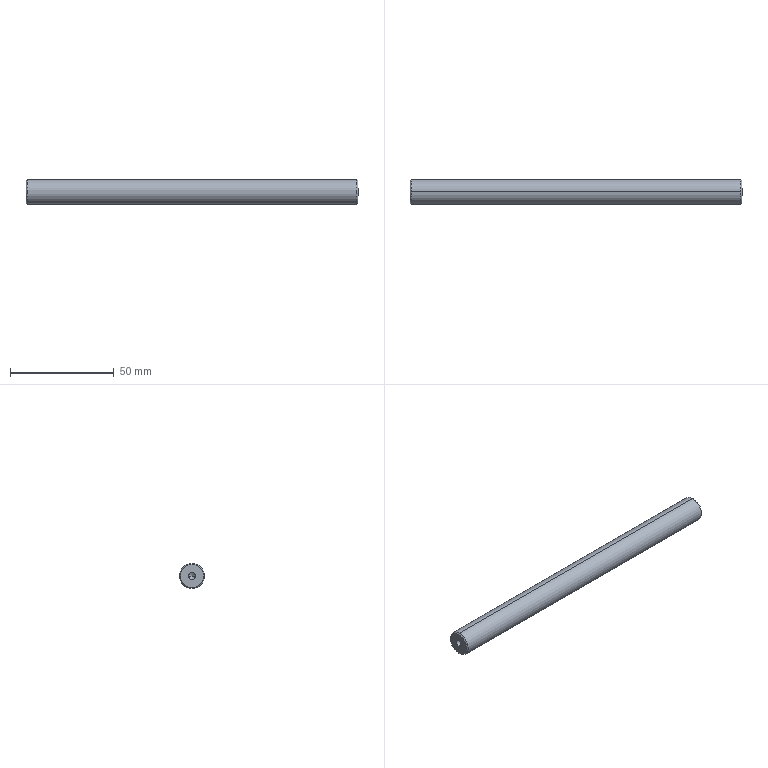Part | STEP file | 12 small shaft 3_SUS304 | 1 solid | 16 faces | box 160 x 12 x 12 mm | volume 17824 mm3 | cone 8 | cylinder 6 | plane 2 | commonest cylinder face diameters 3.3 x4 12 x2
STEP:
#1=CARTESIAN_POINT('',(0.,0.,0.));
#2=DIRECTION('',(0.,0.,1.));
#3=DIRECTION('',(1.,0.,0.));
#4=AXIS2_PLACEMENT_3D('',#1,#2,#3);
#5=CARTESIAN_POINT('',(159.5,0.,6.));
#6=VERTEX_POINT('',#5);
#7=CARTESIAN_POINT('',(159.5,0.,-6.));
#8=VERTEX_POINT('',#7);
#9=CARTESIAN_POINT('',(159.5,0.,0.));
#10=DIRECTION('',(-1.,0.,0.));
#11=DIRECTION('',(0.,0.,1.));
#12=AXIS2_PLACEMENT_3D('',#9,#10,#11);
#13=CIRCLE('',#12,6.);
#14=CARTESIAN_POINT('',(160.,0.,0.));
#15=DIRECTION('',(-1.,0.,0.));
#16=DIRECTION('',(0.,0.,1.));
#17=AXIS2_PLACEMENT_3D('',#14,#15,#16);
#18=CYLINDRICAL_SURFACE('',#17,6.);
#19=CARTESIAN_POINT('',(0.,0.5));
#20=DIRECTION('',(1.,0.));
#21=VECTOR('',#20,1.);
#22=LINE('',#19,#21);
#23=(GEOMETRIC_REPRESENTATION_CONTEXT(2)PARAMETRIC_REPRESENTATION_CONTEXT()REPRESENTATION_CONTEXT('',''));
#24=DEFINITIONAL_REPRESENTATION('',(#22),#23);
#25=PCURVE('',#18,#24);
#26=CARTESIAN_POINT('',(159.5,0.,0.));
#27=DIRECTION('',(-1.,0.,0.));
#28=DIRECTION('',(0.,0.,1.));
#29=AXIS2_PLACEMENT_3D('',#26,#27,#28);
#30=CONICAL_SURFACE('',#29,6.,0.7854);
#31=CARTESIAN_POINT('',(0.,0.));
#32=DIRECTION('',(1.,0.));
#33=VECTOR('',#32,1.);
#34=LINE('',#31,#33);
#35=(GEOMETRIC_REPRESENTATION_CONTEXT(2)PARAMETRIC_REPRESENTATION_CONTEXT()REPRESENTATION_CONTEXT('',''));
#36=DEFINITIONAL_REPRESENTATION('',(#34),#35);
#37=PCURVE('',#30,#36);
#38=SURFACE_CURVE('',#13,(#25,#37),.PCURVE_S1.);
#39=EDGE_CURVE('',#6,#8,#38,.T.);
#40=ORIENTED_EDGE('',*,*,#39,.T.);
#41=CARTESIAN_POINT('',(0.5,0.,-6.));
#42=VERTEX_POINT('',#41);
#43=CARTESIAN_POINT('',(160.,0.,-6.));
#44=DIRECTION('',(-1.,0.,0.));
#45=VECTOR('',#44,1.);
#46=LINE('',#43,#45);
#47=CARTESIAN_POINT('',(3.142,0.));
#48=DIRECTION('',(0.,1.));
#49=VECTOR('',#48,1.);
#50=LINE('',#47,#49);
#51=(GEOMETRIC_REPRESENTATION_CONTEXT(2)PARAMETRIC_REPRESENTATION_CONTEXT()REPRESENTATION_CONTEXT('',''));
#52=DEFINITIONAL_REPRESENTATION('',(#50),#51);
#53=PCURVE('',#18,#52);
#54=CARTESIAN_POINT('',(160.,0.,0.));
#55=DIRECTION('',(-1.,0.,0.));
#56=DIRECTION('',(0.,0.,1.));
#57=AXIS2_PLACEMENT_3D('',#54,#55,#56);
#58=CYLINDRICAL_SURFACE('',#57,6.);
#59=CARTESIAN_POINT('',(3.142,0.));
#60=DIRECTION('',(0.,1.));
#61=VECTOR('',#60,1.);
#62=LINE('',#59,#61);
#63=(GEOMETRIC_REPRESENTATION_CONTEXT(2)PARAMETRIC_REPRESENTATION_CONTEXT()REPRESENTATION_CONTEXT('',''));
#64=DEFINITIONAL_REPRESENTATION('',(#62),#63);
#65=PCURVE('',#58,#64);
#66=SURFACE_CURVE('',#46,(#53,#65),.PCURVE_S1.);
#67=EDGE_CURVE('',#8,#42,#66,.T.);
#68=ORIENTED_EDGE('',*,*,#67,.T.);
#69=CARTESIAN_POINT('',(0.5,0.,6.));
#70=VERTEX_POINT('',#69);
#71=CARTESIAN_POINT('',(0.5,0.,0.));
#72=DIRECTION('',(1.,0.,0.));
#73=DIRECTION('',(0.,0.,1.));
#74=AXIS2_PLACEMENT_3D('',#71,#72,#73);
#75=CIRCLE('',#74,6.);
#76=CARTESIAN_POINT('',(6.283,159.5));
#77=DIRECTION('',(-1.,0.));
#78=VECTOR('',#77,1.);
#79=LINE('',#76,#78);
#80=(GEOMETRIC_REPRESENTATION_CONTEXT(2)PARAMETRIC_REPRESENTATION_CONTEXT()REPRESENTATION_CONTEXT('',''));
#81=DEFINITIONAL_REPRESENTATION('',(#79),#80);
#82=PCURVE('',#18,#81);
#83=CARTESIAN_POINT('',(0.5,0.,0.));
#84=DIRECTION('',(1.,0.,0.));
#85=DIRECTION('',(0.,0.,-1.));
#86=AXIS2_PLACEMENT_3D('',#83,#84,#85);
#87=CONICAL_SURFACE('',#86,6.,0.7854);
#88=CARTESIAN_POINT('',(-3.142,0.));
#89=DIRECTION('',(1.,0.));
#90=VECTOR('',#89,1.);
#91=LINE('',#88,#90);
#92=(GEOMETRIC_REPRESENTATION_CONTEXT(2)PARAMETRIC_REPRESENTATION_CONTEXT()REPRESENTATION_CONTEXT('',''));
#93=DEFINITIONAL_REPRESENTATION('',(#91),#92);
#94=PCURVE('',#87,#93);
#95=SURFACE_CURVE('',#75,(#82,#94),.PCURVE_S1.);
#96=EDGE_CURVE('',#42,#70,#95,.T.);
#97=ORIENTED_EDGE('',*,*,#96,.T.);
#98=CARTESIAN_POINT('',(160.,0.,6.));
#99=DIRECTION('',(-1.,0.,0.));
#100=VECTOR('',#99,1.);
#101=LINE('',#98,#100);
#102=CARTESIAN_POINT('',(0.,0.));
#103=DIRECTION('',(0.,1.));
#104=VECTOR('',#103,1.);
#105=LINE('',#102,#104);
#106=(GEOMETRIC_REPRESENTATION_CONTEXT(2)PARAMETRIC_REPRESENTATION_CONTEXT()REPRESENTATION_CONTEXT('',''));
#107=DEFINITIONAL_REPRESENTATION('',(#105),#106);
#108=PCURVE('',#18,#107);
#109=CARTESIAN_POINT('',(6.283,0.));
#110=DIRECTION('',(0.,1.));
#111=VECTOR('',#110,1.);
#112=LINE('',#109,#111);
#113=(GEOMETRIC_REPRESENTATION_CONTEXT(2)PARAMETRIC_REPRESENTATION_CONTEXT()REPRESENTATION_CONTEXT('',''));
#114=DEFINITIONAL_REPRESENTATION('',(#112),#113);
#115=PCURVE('',#58,#114);
#116=SURFACE_CURVE('',#101,(#108,#115),.PCURVE_S1.);
#117=EDGE_CURVE('',#6,#70,#116,.T.);
#118=ORIENTED_EDGE('',*,*,#117,.F.);
#119=EDGE_LOOP('',(#40,#68,#97,#118));
#120=FACE_BOUND('',#119,.T.);
#121=ADVANCED_FACE('',(#120),#18,.T.);
#122=CARTESIAN_POINT('',(0.,0.,-5.5));
#123=VERTEX_POINT('',#122);
#124=CARTESIAN_POINT('',(0.,0.,5.5));
#125=VERTEX_POINT('',#124);
#126=CARTESIAN_POINT('',(0.,0.,0.));
#127=DIRECTION('',(1.,0.,0.));
#128=DIRECTION('',(0.,0.,-1.));
#129=AXIS2_PLACEMENT_3D('',#126,#127,#128);
#130=CIRCLE('',#129,5.5);
#131=CARTESIAN_POINT('',(0.,-0.5));
#132=DIRECTION('',(1.,0.));
#133=VECTOR('',#132,1.);
#134=LINE('',#131,#133);
#135=(GEOMETRIC_REPRESENTATION_CONTEXT(2)PARAMETRIC_REPRESENTATION_CONTEXT()REPRESENTATION_CONTEXT('',''));
#136=DEFINITIONAL_REPRESENTATION('',(#134),#135);
#137=PCURVE('',#87,#136);
#138=CARTESIAN_POINT('',(0.,0.,0.));
#139=DIRECTION('',(1.,0.,0.));
#140=DIRECTION('',(0.,0.,-1.));
#141=AXIS2_PLACEMENT_3D('',#138,#139,#140);
#142=PLANE('',#141);
#143=CARTESIAN_POINT('',(0.,0.));
#144=DIRECTION('',(1.,0.));
#145=AXIS2_PLACEMENT_2D('',#143,#144);
#146=CIRCLE('',#145,5.5);
#147=(GEOMETRIC_REPRESENTATION_CONTEXT(2)PARAMETRIC_REPRESENTATION_CONTEXT()REPRESENTATION_CONTEXT('',''));
#148=DEFINITIONAL_REPRESENTATION('',(#146),#147);
#149=PCURVE('',#142,#148);
#150=SURFACE_CURVE('',#130,(#137,#149),.PCURVE_S1.);
#151=EDGE_CURVE('',#123,#125,#150,.T.);
#152=ORIENTED_EDGE('',*,*,#151,.T.);
#153=CARTESIAN_POINT('',(0.5,0.,6.));
#154=DIRECTION('',(0.7071,0.,0.7071));
#155=VECTOR('',#154,1.);
#156=LINE('',#153,#155);
#157=CARTESIAN_POINT('',(3.142,0.));
#158=DIRECTION('',(0.,1.));
#159=VECTOR('',#158,1.);
#160=LINE('',#157,#159);
#161=(GEOMETRIC_REPRESENTATION_CONTEXT(2)PARAMETRIC_REPRESENTATION_CONTEXT()REPRESENTATION_CONTEXT('',''));
#162=DEFINITIONAL_REPRESENTATION('',(#160),#161);
#163=PCURVE('',#87,#162);
#164=CARTESIAN_POINT('',(0.5,0.,0.));
#165=DIRECTION('',(1.,0.,0.));
#166=DIRECTION('',(0.,0.,-1.));
#167=AXIS2_PLACEMENT_3D('',#164,#165,#166);
#168=CONICAL_SURFACE('',#167,6.,0.7854);
#169=CARTESIAN_POINT('',(3.142,0.));
#170=DIRECTION('',(0.,1.));
#171=VECTOR('',#170,1.);
#172=LINE('',#169,#171);
#173=(GEOMETRIC_REPRESENTATION_CONTEXT(2)PARAMETRIC_REPRESENTATION_CONTEXT()REPRESENTATION_CONTEXT('',''));
#174=DEFINITIONAL_REPRESENTATION('',(#172),#173);
#175=PCURVE('',#168,#174);
#176=SURFACE_CURVE('',#156,(#163,#175),.PCURVE_S1.);
#177=EDGE_CURVE('',#125,#70,#176,.T.);
#178=ORIENTED_EDGE('',*,*,#177,.T.);
#179=ORIENTED_EDGE('',*,*,#96,.F.);
#180=CARTESIAN_POINT('',(0.5,0.,-6.));
#181=DIRECTION('',(0.7071,0.,-0.7071));
#182=VECTOR('',#181,1.);
#183=LINE('',#180,#182);
#184=CARTESIAN_POINT('',(0.,0.));
#185=DIRECTION('',(0.,1.));
#186=VECTOR('',#185,1.);
#187=LINE('',#184,#186);
#188=(GEOMETRIC_REPRESENTATION_CONTEXT(2)PARAMETRIC_REPRESENTATION_CONTEXT()REPRESENTATION_CONTEXT('',''));
#189=DEFINITIONAL_REPRESENTATION('',(#187),#188);
#190=PCURVE('',#87,#189);
#191=CARTESIAN_POINT('',(6.283,0.));
#192=DIRECTION('',(0.,1.));
#193=VECTOR('',#192,1.);
#194=LINE('',#191,#193);
#195=(GEOMETRIC_REPRESENTATION_CONTEXT(2)PARAMETRIC_REPRESENTATION_CONTEXT()REPRESENTATION_CONTEXT('',''));
#196=DEFINITIONAL_REPRESENTATION('',(#194),#195);
#197=PCURVE('',#168,#196);
#198=SURFACE_CURVE('',#183,(#190,#197),.PCURVE_S1.);
#199=EDGE_CURVE('',#123,#42,#198,.T.);
#200=ORIENTED_EDGE('',*,*,#199,.F.);
#201=EDGE_LOOP('',(#152,#178,#179,#200));
#202=FACE_BOUND('',#201,.T.);
#203=ADVANCED_FACE('',(#202),#87,.T.);
#204=CARTESIAN_POINT('',(160.,0.,5.5));
#205=VERTEX_POINT('',#204);
#206=CARTESIAN_POINT('',(160.,0.,-5.5));
#207=VERTEX_POINT('',#206);
#208=CARTESIAN_POINT('',(160.,0.,0.));
#209=DIRECTION('',(-1.,0.,0.));
#210=DIRECTION('',(0.,0.,1.));
#211=AXIS2_PLACEMENT_3D('',#208,#209,#210);
#212=CIRCLE('',#211,5.5);
#213=CARTESIAN_POINT('',(0.,-0.5));
#214=DIRECTION('',(1.,0.));
#215=VECTOR('',#214,1.);
#216=LINE('',#213,#215);
#217=(GEOMETRIC_REPRESENTATION_CONTEXT(2)PARAMETRIC_REPRESENTATION_CONTEXT()REPRESENTATION_CONTEXT('',''));
#218=DEFINITIONAL_REPRESENTATION('',(#216),#217);
#219=PCURVE('',#30,#218);
#220=CARTESIAN_POINT('',(160.,0.,0.));
#221=DIRECTION('',(1.,0.,0.));
#222=DIRECTION('',(0.,0.,-1.));
#223=AXIS2_PLACEMENT_3D('',#220,#221,#222);
#224=PLANE('',#223);
#225=CARTESIAN_POINT('',(-5.5,0.));
#226=CARTESIAN_POINT('',(-5.5,9.526));
#227=CARTESIAN_POINT('',(2.75,4.763));
#228=CARTESIAN_POINT('',(11.,0.));
#229=CARTESIAN_POINT('',(2.75,-4.763));
#230=CARTESIAN_POINT('',(-5.5,-9.526));
#231=CARTESIAN_POINT('',(-5.5,0.));
#232=(BOUNDED_CURVE()B_SPLINE_CURVE(2,(#225,#226,#227,#228,#229,#230,#231),.UNSPECIFIED.,.T.,.F.)B_SPLINE_CURVE_WITH_KNOTS((1,2,2,2,2,1),(-2.094,0.,2.094,4.189,6.283,8.378),.UNSPECIFIED.)CURVE()GEOMETRIC_REPRESENTATION_ITEM()RATIONAL_B_SPLINE_CURVE((1.,0.5,1.,0.5,1.,0.5,1.))REPRESENTATION_ITEM(''));
#233=(GEOMETRIC_REPRESENTATION_CONTEXT(2)PARAMETRIC_REPRESENTATION_CONTEXT()REPRESENTATION_CONTEXT('',''));
#234=DEFINITIONAL_REPRESENTATION('',(#232),#233);
#235=PCURVE('',#224,#234);
#236=SURFACE_CURVE('',#212,(#219,#235),.PCURVE_S1.);
#237=EDGE_CURVE('',#205,#207,#236,.T.);
#238=ORIENTED_EDGE('',*,*,#237,.T.);
#239=CARTESIAN_POINT('',(159.5,0.,-6.));
#240=DIRECTION('',(-0.7071,0.,-0.7071));
#241=VECTOR('',#240,1.);
#242=LINE('',#239,#241);
#243=CARTESIAN_POINT('',(3.142,0.));
#244=DIRECTION('',(0.,1.));
#245=VECTOR('',#244,1.);
#246=LINE('',#243,#245);
#247=(GEOMETRIC_REPRESENTATION_CONTEXT(2)PARAMETRIC_REPRESENTATION_CONTEXT()REPRESENTATION_CONTEXT('',''));
#248=DEFINITIONAL_REPRESENTATION('',(#246),#247);
#249=PCURVE('',#30,#248);
#250=CARTESIAN_POINT('',(159.5,0.,0.));
#251=DIRECTION('',(-1.,0.,0.));
#252=DIRECTION('',(0.,0.,1.));
#253=AXIS2_PLACEMENT_3D('',#250,#251,#252);
#254=CONICAL_SURFACE('',#253,6.,0.7854);
#255=CARTESIAN_POINT('',(3.142,0.));
#256=DIRECTION('',(0.,1.));
#257=VECTOR('',#256,1.);
#258=LINE('',#255,#257);
#259=(GEOMETRIC_REPRESENTATION_CONTEXT(2)PARAMETRIC_REPRESENTATION_CONTEXT()REPRESENTATION_CONTEXT('',''));
#260=DEFINITIONAL_REPRESENTATION('',(#258),#259);
#261=PCURVE('',#254,#260);
#262=SURFACE_CURVE('',#242,(#249,#261),.PCURVE_S1.);
#263=EDGE_CURVE('',#207,#8,#262,.T.);
#264=ORIENTED_EDGE('',*,*,#263,.T.);
#265=ORIENTED_EDGE('',*,*,#39,.F.);
#266=CARTESIAN_POINT('',(159.5,0.,6.));
#267=DIRECTION('',(-0.7071,0.,0.7071));
#268=VECTOR('',#267,1.);
#269=LINE('',#266,#268);
#270=CARTESIAN_POINT('',(0.,0.));
#271=DIRECTION('',(0.,1.));
#272=VECTOR('',#271,1.);
#273=LINE('',#270,#272);
#274=(GEOMETRIC_REPRESENTATION_CONTEXT(2)PARAMETRIC_REPRESENTATION_CONTEXT()REPRESENTATION_CONTEXT('',''));
#275=DEFINITIONAL_REPRESENTATION('',(#273),#274);
#276=PCURVE('',#30,#275);
#277=CARTESIAN_POINT('',(6.283,0.));
#278=DIRECTION('',(0.,1.));
#279=VECTOR('',#278,1.);
#280=LINE('',#277,#279);
#281=(GEOMETRIC_REPRESENTATION_CONTEXT(2)PARAMETRIC_REPRESENTATION_CONTEXT()REPRESENTATION_CONTEXT('',''));
#282=DEFINITIONAL_REPRESENTATION('',(#280),#281);
#283=PCURVE('',#254,#282);
#284=SURFACE_CURVE('',#269,(#276,#283),.PCURVE_S1.);
#285=EDGE_CURVE('',#205,#6,#284,.T.);
#286=ORIENTED_EDGE('',*,*,#285,.F.);
#287=EDGE_LOOP('',(#238,#264,#265,#286));
#288=FACE_BOUND('',#287,.T.);
#289=ADVANCED_FACE('',(#288),#30,.T.);
#290=CARTESIAN_POINT('',(14.5,-1.65,0.));
#291=VERTEX_POINT('',#290);
#292=CARTESIAN_POINT('',(14.5,0.,1.65));
#293=VERTEX_POINT('',#292);
#294=CARTESIAN_POINT('',(14.5,0.,0.));
#295=DIRECTION('',(-1.,0.,0.));
#296=DIRECTION('',(0.,0.,1.));
#297=AXIS2_PLACEMENT_3D('',#294,#295,#296);
#298=CIRCLE('',#297,1.65);
#299=CARTESIAN_POINT('',(0.,0.,0.));
#300=DIRECTION('',(-1.,0.,0.));
#301=DIRECTION('',(0.,0.,1.));
#302=AXIS2_PLACEMENT_3D('',#299,#300,#301);
#303=CYLINDRICAL_SURFACE('',#302,1.65);
#304=CARTESIAN_POINT('',(0.,-14.5));
#305=DIRECTION('',(1.,0.));
#306=VECTOR('',#305,1.);
#307=LINE('',#304,#306);
#308=(GEOMETRIC_REPRESENTATION_CONTEXT(2)PARAMETRIC_REPRESENTATION_CONTEXT()REPRESENTATION_CONTEXT('',''));
#309=DEFINITIONAL_REPRESENTATION('',(#307),#308);
#310=PCURVE('',#303,#309);
#311=CARTESIAN_POINT('',(14.5,0.,0.));
#312=DIRECTION('',(-1.,0.,0.));
#313=DIRECTION('',(0.,-1.,0.));
#314=AXIS2_PLACEMENT_3D('',#311,#312,#313);
#315=CONICAL_SURFACE('',#314,1.65,1.03);
#316=CARTESIAN_POINT('',(-4.712,0.));
#317=DIRECTION('',(1.,0.));
#318=VECTOR('',#317,1.);
#319=LINE('',#316,#318);
#320=(GEOMETRIC_REPRESENTATION_CONTEXT(2)PARAMETRIC_REPRESENTATION_CONTEXT()REPRESENTATION_CONTEXT('',''));
#321=DEFINITIONAL_REPRESENTATION('',(#319),#320);
#322=PCURVE('',#315,#321);
#323=SURFACE_CURVE('',#298,(#310,#322),.PCURVE_S1.);
#324=EDGE_CURVE('',#291,#293,#323,.T.);
#325=ORIENTED_EDGE('',*,*,#324,.T.);
#326=CARTESIAN_POINT('',(0.,0.,1.65));
#327=VERTEX_POINT('',#326);
#328=CARTESIAN_POINT('',(0.,0.,1.65));
#329=DIRECTION('',(-1.,0.,0.));
#330=VECTOR('',#329,1.);
#331=LINE('',#328,#330);
#332=CARTESIAN_POINT('',(6.283,0.));
#333=DIRECTION('',(0.,1.));
#334=VECTOR('',#333,1.);
#335=LINE('',#332,#334);
#336=(GEOMETRIC_REPRESENTATION_CONTEXT(2)PARAMETRIC_REPRESENTATION_CONTEXT()REPRESENTATION_CONTEXT('',''));
#337=DEFINITIONAL_REPRESENTATION('',(#335),#336);
#338=PCURVE('',#303,#337);
#339=CARTESIAN_POINT('',(0.,0.,0.));
#340=DIRECTION('',(-1.,0.,0.));
#341=DIRECTION('',(0.,0.,1.));
#342=AXIS2_PLACEMENT_3D('',#339,#340,#341);
#343=CYLINDRICAL_SURFACE('',#342,1.65);
#344=CARTESIAN_POINT('',(0.,0.));
#345=DIRECTION('',(0.,1.));
#346=VECTOR('',#345,1.);
#347=LINE('',#344,#346);
#348=(GEOMETRIC_REPRESENTATION_CONTEXT(2)PARAMETRIC_REPRESENTATION_CONTEXT()REPRESENTATION_CONTEXT('',''));
#349=DEFINITIONAL_REPRESENTATION('',(#347),#348);
#350=PCURVE('',#343,#349);
#351=SURFACE_CURVE('',#331,(#338,#350),.PCURVE_S1.);
#352=EDGE_CURVE('',#293,#327,#351,.T.);
#353=ORIENTED_EDGE('',*,*,#352,.T.);
#354=CARTESIAN_POINT('',(0.,0.,-1.65));
#355=VERTEX_POINT('',#354);
#356=CARTESIAN_POINT('',(0.,0.,0.));
#357=DIRECTION('',(-1.,0.,0.));
#358=DIRECTION('',(0.,0.,1.));
#359=AXIS2_PLACEMENT_3D('',#356,#357,#358);
#360=CIRCLE('',#359,1.65);
#361=CARTESIAN_POINT('',(0.,0.));
#362=DIRECTION('',(1.,0.));
#363=VECTOR('',#362,1.);
#364=LINE('',#361,#363);
#365=(GEOMETRIC_REPRESENTATION_CONTEXT(2)PARAMETRIC_REPRESENTATION_CONTEXT()REPRESENTATION_CONTEXT('',''));
#366=DEFINITIONAL_REPRESENTATION('',(#364),#365);
#367=PCURVE('',#303,#366);
#368=CARTESIAN_POINT('',(-1.65,0.));
#369=CARTESIAN_POINT('',(-1.65,2.858));
#370=CARTESIAN_POINT('',(0.825,1.429));
#371=CARTESIAN_POINT('',(3.3,0.));
#372=CARTESIAN_POINT('',(0.825,-1.429));
#373=CARTESIAN_POINT('',(-1.65,-2.858));
#374=CARTESIAN_POINT('',(-1.65,0.));
#375=(BOUNDED_CURVE()B_SPLINE_CURVE(2,(#368,#369,#370,#371,#372,#373,#374),.UNSPECIFIED.,.T.,.F.)B_SPLINE_CURVE_WITH_KNOTS((1,2,2,2,2,1),(-2.094,0.,2.094,4.189,6.283,8.378),.UNSPECIFIED.)CURVE()GEOMETRIC_REPRESENTATION_ITEM()RATIONAL_B_SPLINE_CURVE((1.,0.5,1.,0.5,1.,0.5,1.))REPRESENTATION_ITEM(''));
#376=(GEOMETRIC_REPRESENTATION_CONTEXT(2)PARAMETRIC_REPRESENTATION_CONTEXT()REPRESENTATION_CONTEXT('',''));
#377=DEFINITIONAL_REPRESENTATION('',(#375),#376);
#378=PCURVE('',#142,#377);
#379=SURFACE_CURVE('',#360,(#367,#378),.PCURVE_S1.);
#380=EDGE_CURVE('',#355,#327,#379,.T.);
#381=ORIENTED_EDGE('',*,*,#380,.F.);
#382=CARTESIAN_POINT('',(14.5,0.,-1.65));
#383=VERTEX_POINT('',#382);
#384=CARTESIAN_POINT('',(0.,0.,-1.65));
#385=DIRECTION('',(-1.,0.,0.));
#386=VECTOR('',#385,1.);
#387=LINE('',#384,#386);
#388=CARTESIAN_POINT('',(3.142,0.));
#389=DIRECTION('',(0.,1.));
#390=VECTOR('',#389,1.);
#391=LINE('',#388,#390);
#392=(GEOMETRIC_REPRESENTATION_CONTEXT(2)PARAMETRIC_REPRESENTATION_CONTEXT()REPRESENTATION_CONTEXT('',''));
#393=DEFINITIONAL_REPRESENTATION('',(#391),#392);
#394=PCURVE('',#303,#393);
#395=CARTESIAN_POINT('',(3.142,0.));
#396=DIRECTION('',(0.,1.));
#397=VECTOR('',#396,1.);
#398=LINE('',#395,#397);
#399=(GEOMETRIC_REPRESENTATION_CONTEXT(2)PARAMETRIC_REPRESENTATION_CONTEXT()REPRESENTATION_CONTEXT('',''));
#400=DEFINITIONAL_REPRESENTATION('',(#398),#399);
#401=PCURVE('',#343,#400);
#402=SURFACE_CURVE('',#387,(#394,#401),.PCURVE_S1.);
#403=EDGE_CURVE('',#383,#355,#402,.T.);
#404=ORIENTED_EDGE('',*,*,#403,.F.);
#405=CARTESIAN_POINT('',(14.5,0.,0.));
#406=DIRECTION('',(-1.,0.,0.));
#407=DIRECTION('',(0.,0.,1.));
#408=AXIS2_PLACEMENT_3D('',#405,#406,#407);
#409=CIRCLE('',#408,1.65);
#410=CARTESIAN_POINT('',(0.,-14.5));
#411=DIRECTION('',(1.,0.));
#412=VECTOR('',#411,1.);
#413=LINE('',#410,#412);
#414=(GEOMETRIC_REPRESENTATION_CONTEXT(2)PARAMETRIC_REPRESENTATION_CONTEXT()REPRESENTATION_CONTEXT('',''));
#415=DEFINITIONAL_REPRESENTATION('',(#413),#414);
#416=PCURVE('',#303,#415);
#417=CARTESIAN_POINT('',(14.5,0.,0.));
#418=DIRECTION('',(-1.,0.,0.));
#419=DIRECTION('',(0.,-1.,0.));
#420=AXIS2_PLACEMENT_3D('',#417,#418,#419);
#421=CONICAL_SURFACE('',#420,1.65,1.03);
#422=CARTESIAN_POINT('',(1.571,0.));
#423=DIRECTION('',(1.,0.));
#424=VECTOR('',#423,1.);
#425=LINE('',#422,#424);
#426=(GEOMETRIC_REPRESENTATION_CONTEXT(2)PARAMETRIC_REPRESENTATION_CONTEXT()REPRESENTATION_CONTEXT('',''));
#427=DEFINITIONAL_REPRESENTATION('',(#425),#426);
#428=PCURVE('',#421,#427);
#429=SURFACE_CURVE('',#409,(#416,#428),.PCURVE_S1.);
#430=EDGE_CURVE('',#383,#291,#429,.T.);
#431=ORIENTED_EDGE('',*,*,#430,.T.);
#432=EDGE_LOOP('',(#325,#353,#381,#404,#431));
#433=FACE_BOUND('',#432,.F.);
#434=ADVANCED_FACE('',(#433),#303,.F.);
#435=CARTESIAN_POINT('',(144.5,0.,-1.65));
#436=VERTEX_POINT('',#435);
#437=CARTESIAN_POINT('',(160.,0.,-1.65));
#438=VERTEX_POINT('',#437);
#439=CARTESIAN_POINT('',(160.,0.,-1.65));
#440=DIRECTION('',(1.,0.,0.));
#441=VECTOR('',#440,1.);
#442=LINE('',#439,#441);
#443=CARTESIAN_POINT('',(160.,0.,0.));
#444=DIRECTION('',(1.,0.,0.));
#445=DIRECTION('',(0.,0.,-1.));
#446=AXIS2_PLACEMENT_3D('',#443,#444,#445);
#447=CYLINDRICAL_SURFACE('',#446,1.65);
#448=CARTESIAN_POINT('',(6.283,0.));
#449=DIRECTION('',(0.,1.));
#450=VECTOR('',#449,1.);
#451=LINE('',#448,#450);
#452=(GEOMETRIC_REPRESENTATION_CONTEXT(2)PARAMETRIC_REPRESENTATION_CONTEXT()REPRESENTATION_CONTEXT('',''));
#453=DEFINITIONAL_REPRESENTATION('',(#451),#452);
#454=PCURVE('',#447,#453);
#455=CARTESIAN_POINT('',(160.,0.,0.));
#456=DIRECTION('',(1.,0.,0.));
#457=DIRECTION('',(0.,0.,-1.));
#458=AXIS2_PLACEMENT_3D('',#455,#456,#457);
#459=CYLINDRICAL_SURFACE('',#458,1.65);
#460=CARTESIAN_POINT('',(0.,0.));
#461=DIRECTION('',(0.,1.));
#462=VECTOR('',#461,1.);
#463=LINE('',#460,#462);
#464=(GEOMETRIC_REPRESENTATION_CONTEXT(2)PARAMETRIC_REPRESENTATION_CONTEXT()REPRESENTATION_CONTEXT('',''));
#465=DEFINITIONAL_REPRESENTATION('',(#463),#464);
#466=PCURVE('',#459,#465);
#467=SURFACE_CURVE('',#442,(#454,#466),.PCURVE_S1.);
#468=EDGE_CURVE('',#436,#438,#467,.T.);
#469=ORIENTED_EDGE('',*,*,#468,.T.);
#470=CARTESIAN_POINT('',(160.,0.,1.65));
#471=VERTEX_POINT('',#470);
#472=CARTESIAN_POINT('',(160.,0.,0.));
#473=DIRECTION('',(-1.,0.,0.));
#474=DIRECTION('',(0.,0.,-1.));
#475=AXIS2_PLACEMENT_3D('',#472,#473,#474);
#476=CIRCLE('',#475,1.65);
#477=CARTESIAN_POINT('',(6.283,0.));
#478=DIRECTION('',(-1.,0.));
#479=VECTOR('',#478,1.);
#480=LINE('',#477,#479);
#481=(GEOMETRIC_REPRESENTATION_CONTEXT(2)PARAMETRIC_REPRESENTATION_CONTEXT()REPRESENTATION_CONTEXT('',''));
#482=DEFINITIONAL_REPRESENTATION('',(#480),#481);
#483=PCURVE('',#447,#482);
#484=CARTESIAN_POINT('',(1.65,0.));
#485=CARTESIAN_POINT('',(1.65,-2.858));
#486=CARTESIAN_POINT('',(-0.825,-1.429));
#487=CARTESIAN_POINT('',(-3.3,0.));
#488=CARTESIAN_POINT('',(-0.825,1.429));
#489=CARTESIAN_POINT('',(1.65,2.858));
#490=CARTESIAN_POINT('',(1.65,0.));
#491=(BOUNDED_CURVE()B_SPLINE_CURVE(2,(#484,#485,#486,#487,#488,#489,#490),.UNSPECIFIED.,.T.,.F.)B_SPLINE_CURVE_WITH_KNOTS((1,2,2,2,2,1),(-2.094,0.,2.094,4.189,6.283,8.378),.UNSPECIFIED.)CURVE()GEOMETRIC_REPRESENTATION_ITEM()RATIONAL_B_SPLINE_CURVE((1.,0.5,1.,0.5,1.,0.5,1.))REPRESENTATION_ITEM(''));
#492=(GEOMETRIC_REPRESENTATION_CONTEXT(2)PARAMETRIC_REPRESENTATION_CONTEXT()REPRESENTATION_CONTEXT('',''));
#493=DEFINITIONAL_REPRESENTATION('',(#491),#492);
#494=PCURVE('',#224,#493);
#495=SURFACE_CURVE('',#476,(#483,#494),.PCURVE_S1.);
#496=EDGE_CURVE('',#438,#471,#495,.T.);
#497=ORIENTED_EDGE('',*,*,#496,.T.);
#498=CARTESIAN_POINT('',(144.5,0.,1.65));
#499=VERTEX_POINT('',#498);
#500=CARTESIAN_POINT('',(160.,0.,1.65));
#501=DIRECTION('',(1.,0.,0.));
#502=VECTOR('',#501,1.);
#503=LINE('',#500,#502);
#504=CARTESIAN_POINT('',(3.142,0.));
#505=DIRECTION('',(0.,1.));
#506=VECTOR('',#505,1.);
#507=LINE('',#504,#506);
#508=(GEOMETRIC_REPRESENTATION_CONTEXT(2)PARAMETRIC_REPRESENTATION_CONTEXT()REPRESENTATION_CONTEXT('',''));
#509=DEFINITIONAL_REPRESENTATION('',(#507),#508);
#510=PCURVE('',#447,#509);
#511=CARTESIAN_POINT('',(3.142,0.));
#512=DIRECTION('',(0.,1.));
#513=VECTOR('',#512,1.);
#514=LINE('',#511,#513);
#515=(GEOMETRIC_REPRESENTATION_CONTEXT(2)PARAMETRIC_REPRESENTATION_CONTEXT()REPRESENTATION_CONTEXT('',''));
#516=DEFINITIONAL_REPRESENTATION('',(#514),#515);
#517=PCURVE('',#459,#516);
#518=SURFACE_CURVE('',#503,(#510,#517),.PCURVE_S1.);
#519=EDGE_CURVE('',#499,#471,#518,.T.);
#520=ORIENTED_EDGE('',*,*,#519,.F.);
#521=CARTESIAN_POINT('',(144.5,0.,0.));
#522=DIRECTION('',(1.,0.,0.));
#523=DIRECTION('',(0.,0.,-1.));
#524=AXIS2_PLACEMENT_3D('',#521,#522,#523);
#525=CIRCLE('',#524,1.65);
#526=CARTESIAN_POINT('',(0.,-15.5));
#527=DIRECTION('',(1.,0.));
#528=VECTOR('',#527,1.);
#529=LINE('',#526,#528);
#530=(GEOMETRIC_REPRESENTATION_CONTEXT(2)PARAMETRIC_REPRESENTATION_CONTEXT()REPRESENTATION_CONTEXT('',''));
#531=DEFINITIONAL_REPRESENTATION('',(#529),#530);
#532=PCURVE('',#447,#531);
#533=CARTESIAN_POINT('',(144.5,0.,0.));
#534=DIRECTION('',(1.,0.,0.));
#535=DIRECTION('',(0.,0.,-1.));
#536=AXIS2_PLACEMENT_3D('',#533,#534,#535);
#537=CONICAL_SURFACE('',#536,1.65,1.03);
#538=CARTESIAN_POINT('',(0.,0.));
#539=DIRECTION('',(1.,0.));
#540=VECTOR('',#539,1.);
#541=LINE('',#538,#540);
#542=(GEOMETRIC_REPRESENTATION_CONTEXT(2)PARAMETRIC_REPRESENTATION_CONTEXT()REPRESENTATION_CONTEXT('',''));
#543=DEFINITIONAL_REPRESENTATION('',(#541),#542);
#544=PCURVE('',#537,#543);
#545=SURFACE_CURVE('',#525,(#532,#544),.PCURVE_S1.);
#546=EDGE_CURVE('',#499,#436,#545,.T.);
#547=ORIENTED_EDGE('',*,*,#546,.T.);
#548=EDGE_LOOP('',(#469,#497,#520,#547));
#549=FACE_BOUND('',#548,.F.);
#550=ADVANCED_FACE('',(#549),#447,.F.);
#551=ORIENTED_EDGE('',*,*,#430,.F.);
#552=CARTESIAN_POINT('',(14.5,1.65,0.));
#553=VERTEX_POINT('',#552);
#554=CARTESIAN_POINT('',(14.5,0.,0.));
#555=DIRECTION('',(-1.,0.,0.));
#556=DIRECTION('',(0.,0.,1.));
#557=AXIS2_PLACEMENT_3D('',#554,#555,#556);
#558=CIRCLE('',#557,1.65);
#559=CARTESIAN_POINT('',(1.571,0.));
#560=DIRECTION('',(1.,0.));
#561=VECTOR('',#560,1.);
#562=LINE('',#559,#561);
#563=(GEOMETRIC_REPRESENTATION_CONTEXT(2)PARAMETRIC_REPRESENTATION_CONTEXT()REPRESENTATION_CONTEXT('',''));
#564=DEFINITIONAL_REPRESENTATION('',(#562),#563);
#565=PCURVE('',#421,#564);
#566=CARTESIAN_POINT('',(0.,-14.5));
#567=DIRECTION('',(1.,0.));
#568=VECTOR('',#567,1.);
#569=LINE('',#566,#568);
#570=(GEOMETRIC_REPRESENTATION_CONTEXT(2)PARAMETRIC_REPRESENTATION_CONTEXT()REPRESENTATION_CONTEXT('',''));
#571=DEFINITIONAL_REPRESENTATION('',(#569),#570);
#572=PCURVE('',#343,#571);
#573=SURFACE_CURVE('',#558,(#565,#572),.PCURVE_S1.);
#574=EDGE_CURVE('',#553,#383,#573,.T.);
#575=ORIENTED_EDGE('',*,*,#574,.F.);
#576=CARTESIAN_POINT('',(15.491,0.,0.));
#577=VERTEX_POINT('',#576);
#578=CARTESIAN_POINT('',(14.5,1.65,0.));
#579=DIRECTION('',(-0.515,0.8572,0.));
#580=VECTOR('',#579,1.);
#581=LINE('',#578,#580);
#582=CARTESIAN_POINT('',(3.142,0.));
#583=DIRECTION('',(0.,1.));
#584=VECTOR('',#583,1.);
#585=LINE('',#582,#584);
#586=(GEOMETRIC_REPRESENTATION_CONTEXT(2)PARAMETRIC_REPRESENTATION_CONTEXT()REPRESENTATION_CONTEXT('',''));
#587=DEFINITIONAL_REPRESENTATION('',(#585),#586);
#588=PCURVE('',#421,#587);
#589=CARTESIAN_POINT('',(3.142,0.));
#590=DIRECTION('',(0.,1.));
#591=VECTOR('',#590,1.);
#592=LINE('',#589,#591);
#593=(GEOMETRIC_REPRESENTATION_CONTEXT(2)PARAMETRIC_REPRESENTATION_CONTEXT()REPRESENTATION_CONTEXT('',''));
#594=DEFINITIONAL_REPRESENTATION('',(#592),#593);
#595=PCURVE('',#315,#594);
#596=SURFACE_CURVE('',#581,(#588,#595),.PCURVE_S1.);
#597=EDGE_CURVE('',#577,#553,#596,.T.);
#598=ORIENTED_EDGE('',*,*,#597,.F.);
#599=CARTESIAN_POINT('',(14.5,-1.65,0.));
#600=DIRECTION('',(-0.515,-0.8572,0.));
#601=VECTOR('',#600,1.);
#602=LINE('',#599,#601);
#603=CARTESIAN_POINT('',(6.283,0.));
#604=DIRECTION('',(0.,1.));
#605=VECTOR('',#604,1.);
#606=LINE('',#603,#605);
#607=(GEOMETRIC_REPRESENTATION_CONTEXT(2)PARAMETRIC_REPRESENTATION_CONTEXT()REPRESENTATION_CONTEXT('',''));
#608=DEFINITIONAL_REPRESENTATION('',(#606),#607);
#609=PCURVE('',#421,#608);
#610=CARTESIAN_POINT('',(0.,0.));
#611=DIRECTION('',(0.,1.));
#612=VECTOR('',#611,1.);
#613=LINE('',#610,#612);
#614=(GEOMETRIC_REPRESENTATION_CONTEXT(2)PARAMETRIC_REPRESENTATION_CONTEXT()REPRESENTATION_CONTEXT('',''));
#615=DEFINITIONAL_REPRESENTATION('',(#613),#614);
#616=PCURVE('',#315,#615);
#617=SURFACE_CURVE('',#602,(#609,#616),.PCURVE_S1.);
#618=EDGE_CURVE('',#577,#291,#617,.T.);
#619=ORIENTED_EDGE('',*,*,#618,.T.);
#620=EDGE_LOOP('',(#551,#575,#598,#619));
#621=FACE_BOUND('',#620,.F.);
#622=ADVANCED_FACE('',(#621),#421,.F.);
#623=ORIENTED_EDGE('',*,*,#546,.F.);
#624=CARTESIAN_POINT('',(143.509,0.,0.));
#625=VERTEX_POINT('',#624);
#626=CARTESIAN_POINT('',(144.5,0.,1.65));
#627=DIRECTION('',(0.515,0.,0.8572));
#628=VECTOR('',#627,1.);
#629=LINE('',#626,#628);
#630=CARTESIAN_POINT('',(3.142,0.));
#631=DIRECTION('',(0.,1.));
#632=VECTOR('',#631,1.);
#633=LINE('',#630,#632);
#634=(GEOMETRIC_REPRESENTATION_CONTEXT(2)PARAMETRIC_REPRESENTATION_CONTEXT()REPRESENTATION_CONTEXT('',''));
#635=DEFINITIONAL_REPRESENTATION('',(#633),#634);
#636=PCURVE('',#537,#635);
#637=CARTESIAN_POINT('',(144.5,0.,0.));
#638=DIRECTION('',(1.,0.,0.));
#639=DIRECTION('',(0.,0.,-1.));
#640=AXIS2_PLACEMENT_3D('',#637,#638,#639);
#641=CONICAL_SURFACE('',#640,1.65,1.03);
#642=CARTESIAN_POINT('',(3.142,0.));
#643=DIRECTION('',(0.,1.));
#644=VECTOR('',#643,1.);
#645=LINE('',#642,#644);
#646=(GEOMETRIC_REPRESENTATION_CONTEXT(2)PARAMETRIC_REPRESENTATION_CONTEXT()REPRESENTATION_CONTEXT('',''));
#647=DEFINITIONAL_REPRESENTATION('',(#645),#646);
#648=PCURVE('',#641,#647);
#649=SURFACE_CURVE('',#629,(#636,#648),.PCURVE_S1.);
#650=EDGE_CURVE('',#625,#499,#649,.T.);
#651=ORIENTED_EDGE('',*,*,#650,.F.);
#652=CARTESIAN_POINT('',(144.5,0.,-1.65));
#653=DIRECTION('',(0.515,0.,-0.8572));
#654=VECTOR('',#653,1.);
#655=LINE('',#652,#654);
#656=CARTESIAN_POINT('',(6.283,0.));
#657=DIRECTION('',(0.,1.));
#658=VECTOR('',#657,1.);
#659=LINE('',#656,#658);
#660=(GEOMETRIC_REPRESENTATION_CONTEXT(2)PARAMETRIC_REPRESENTATION_CONTEXT()REPRESENTATION_CONTEXT('',''));
#661=DEFINITIONAL_REPRESENTATION('',(#659),#660);
#662=PCURVE('',#537,#661);
#663=CARTESIAN_POINT('',(0.,0.));
#664=DIRECTION('',(0.,1.));
#665=VECTOR('',#664,1.);
#666=LINE('',#663,#665);
#667=(GEOMETRIC_REPRESENTATION_CONTEXT(2)PARAMETRIC_REPRESENTATION_CONTEXT()REPRESENTATION_CONTEXT('',''));
#668=DEFINITIONAL_REPRESENTATION('',(#666),#667);
#669=PCURVE('',#641,#668);
#670=SURFACE_CURVE('',#655,(#662,#669),.PCURVE_S1.);
#671=EDGE_CURVE('',#625,#436,#670,.T.);
#672=ORIENTED_EDGE('',*,*,#671,.T.);
#673=EDGE_LOOP('',(#623,#651,#672));
#674=FACE_BOUND('',#673,.F.);
#675=ADVANCED_FACE('',(#674),#537,.F.);
#676=ORIENTED_EDGE('',*,*,#67,.F.);
#677=CARTESIAN_POINT('',(159.5,0.,0.));
#678=DIRECTION('',(-1.,0.,0.));
#679=DIRECTION('',(0.,0.,1.));
#680=AXIS2_PLACEMENT_3D('',#677,#678,#679);
#681=CIRCLE('',#680,6.);
#682=CARTESIAN_POINT('',(0.,0.5));
#683=DIRECTION('',(1.,0.));
#684=VECTOR('',#683,1.);
#685=LINE('',#682,#684);
#686=(GEOMETRIC_REPRESENTATION_CONTEXT(2)PARAMETRIC_REPRESENTATION_CONTEXT()REPRESENTATION_CONTEXT('',''));
#687=DEFINITIONAL_REPRESENTATION('',(#685),#686);
#688=PCURVE('',#58,#687);
#689=CARTESIAN_POINT('',(0.,0.));
#690=DIRECTION('',(1.,0.));
#691=VECTOR('',#690,1.);
#692=LINE('',#689,#691);
#693=(GEOMETRIC_REPRESENTATION_CONTEXT(2)PARAMETRIC_REPRESENTATION_CONTEXT()REPRESENTATION_CONTEXT('',''));
#694=DEFINITIONAL_REPRESENTATION('',(#692),#693);
#695=PCURVE('',#254,#694);
#696=SURFACE_CURVE('',#681,(#688,#695),.PCURVE_S1.);
#697=EDGE_CURVE('',#8,#6,#696,.T.);
#698=ORIENTED_EDGE('',*,*,#697,.T.);
#699=ORIENTED_EDGE('',*,*,#117,.T.);
#700=CARTESIAN_POINT('',(0.5,0.,0.));
#701=DIRECTION('',(1.,0.,0.));
#702=DIRECTION('',(0.,0.,1.));
#703=AXIS2_PLACEMENT_3D('',#700,#701,#702);
#704=CIRCLE('',#703,6.);
#705=CARTESIAN_POINT('',(6.283,159.5));
#706=DIRECTION('',(-1.,0.));
#707=VECTOR('',#706,1.);
#708=LINE('',#705,#707);
#709=(GEOMETRIC_REPRESENTATION_CONTEXT(2)PARAMETRIC_REPRESENTATION_CONTEXT()REPRESENTATION_CONTEXT('',''));
#710=DEFINITIONAL_REPRESENTATION('',(#708),#709);
#711=PCURVE('',#58,#710);
#712=CARTESIAN_POINT('',(3.142,0.));
#713=DIRECTION('',(1.,0.));
#714=VECTOR('',#713,1.);
#715=LINE('',#712,#714);
#716=(GEOMETRIC_REPRESENTATION_CONTEXT(2)PARAMETRIC_REPRESENTATION_CONTEXT()REPRESENTATION_CONTEXT('',''));
#717=DEFINITIONAL_REPRESENTATION('',(#715),#716);
#718=PCURVE('',#168,#717);
#719=SURFACE_CURVE('',#704,(#711,#718),.PCURVE_S1.);
#720=EDGE_CURVE('',#70,#42,#719,.T.);
#721=ORIENTED_EDGE('',*,*,#720,.T.);
#722=EDGE_LOOP('',(#676,#698,#699,#721));
#723=FACE_BOUND('',#722,.T.);
#724=ADVANCED_FACE('',(#723),#58,.T.);
#725=ORIENTED_EDGE('',*,*,#177,.F.);
#726=CARTESIAN_POINT('',(0.,0.,0.));
#727=DIRECTION('',(1.,0.,0.));
#728=DIRECTION('',(0.,0.,-1.));
#729=AXIS2_PLACEMENT_3D('',#726,#727,#728);
#730=CIRCLE('',#729,5.5);
#731=CARTESIAN_POINT('',(0.,-0.5));
#732=DIRECTION('',(1.,0.));
#733=VECTOR('',#732,1.);
#734=LINE('',#731,#733);
#735=(GEOMETRIC_REPRESENTATION_CONTEXT(2)PARAMETRIC_REPRESENTATION_CONTEXT()REPRESENTATION_CONTEXT('',''));
#736=DEFINITIONAL_REPRESENTATION('',(#734),#735);
#737=PCURVE('',#168,#736);
#738=CARTESIAN_POINT('',(0.,0.));
#739=DIRECTION('',(1.,0.));
#740=AXIS2_PLACEMENT_2D('',#738,#739);
#741=CIRCLE('',#740,5.5);
#742=(GEOMETRIC_REPRESENTATION_CONTEXT(2)PARAMETRIC_REPRESENTATION_CONTEXT()REPRESENTATION_CONTEXT('',''));
#743=DEFINITIONAL_REPRESENTATION('',(#741),#742);
#744=PCURVE('',#142,#743);
#745=SURFACE_CURVE('',#730,(#737,#744),.PCURVE_S1.);
#746=EDGE_CURVE('',#125,#123,#745,.T.);
#747=ORIENTED_EDGE('',*,*,#746,.T.);
#748=ORIENTED_EDGE('',*,*,#199,.T.);
#749=ORIENTED_EDGE('',*,*,#720,.F.);
#750=EDGE_LOOP('',(#725,#747,#748,#749));
#751=FACE_BOUND('',#750,.T.);
#752=ADVANCED_FACE('',(#751),#168,.T.);
#753=ORIENTED_EDGE('',*,*,#263,.F.);
#754=CARTESIAN_POINT('',(160.,0.,0.));
#755=DIRECTION('',(-1.,0.,0.));
#756=DIRECTION('',(0.,0.,1.));
#757=AXIS2_PLACEMENT_3D('',#754,#755,#756);
#758=CIRCLE('',#757,5.5);
#759=CARTESIAN_POINT('',(0.,-0.5));
#760=DIRECTION('',(1.,0.));
#761=VECTOR('',#760,1.);
#762=LINE('',#759,#761);
#763=(GEOMETRIC_REPRESENTATION_CONTEXT(2)PARAMETRIC_REPRESENTATION_CONTEXT()REPRESENTATION_CONTEXT('',''));
#764=DEFINITIONAL_REPRESENTATION('',(#762),#763);
#765=PCURVE('',#254,#764);
#766=CARTESIAN_POINT('',(-5.5,0.));
#767=CARTESIAN_POINT('',(-5.5,9.526));
#768=CARTESIAN_POINT('',(2.75,4.763));
#769=CARTESIAN_POINT('',(11.,0.));
#770=CARTESIAN_POINT('',(2.75,-4.763));
#771=CARTESIAN_POINT('',(-5.5,-9.526));
#772=CARTESIAN_POINT('',(-5.5,0.));
#773=(BOUNDED_CURVE()B_SPLINE_CURVE(2,(#766,#767,#768,#769,#770,#771,#772),.UNSPECIFIED.,.T.,.F.)B_SPLINE_CURVE_WITH_KNOTS((1,2,2,2,2,1),(-2.094,0.,2.094,4.189,6.283,8.378),.UNSPECIFIED.)CURVE()GEOMETRIC_REPRESENTATION_ITEM()RATIONAL_B_SPLINE_CURVE((1.,0.5,1.,0.5,1.,0.5,1.))REPRESENTATION_ITEM(''));
#774=(GEOMETRIC_REPRESENTATION_CONTEXT(2)PARAMETRIC_REPRESENTATION_CONTEXT()REPRESENTATION_CONTEXT('',''));
#775=DEFINITIONAL_REPRESENTATION('',(#773),#774);
#776=PCURVE('',#224,#775);
#777=SURFACE_CURVE('',#758,(#765,#776),.PCURVE_S1.);
#778=EDGE_CURVE('',#207,#205,#777,.T.);
#779=ORIENTED_EDGE('',*,*,#778,.T.);
#780=ORIENTED_EDGE('',*,*,#285,.T.);
#781=ORIENTED_EDGE('',*,*,#697,.F.);
#782=EDGE_LOOP('',(#753,#779,#780,#781));
#783=FACE_BOUND('',#782,.T.);
#784=ADVANCED_FACE('',(#783),#254,.T.);
#785=ORIENTED_EDGE('',*,*,#151,.F.);
#786=ORIENTED_EDGE('',*,*,#746,.F.);
#787=EDGE_LOOP('',(#785,#786));
#788=FACE_BOUND('',#787,.T.);
#789=CARTESIAN_POINT('',(0.,0.,0.));
#790=DIRECTION('',(-1.,0.,0.));
#791=DIRECTION('',(0.,0.,1.));
#792=AXIS2_PLACEMENT_3D('',#789,#790,#791);
#793=CIRCLE('',#792,1.65);
#794=CARTESIAN_POINT('',(-1.65,0.));
#795=CARTESIAN_POINT('',(-1.65,2.858));
#796=CARTESIAN_POINT('',(0.825,1.429));
#797=CARTESIAN_POINT('',(3.3,0.));
#798=CARTESIAN_POINT('',(0.825,-1.429));
#799=CARTESIAN_POINT('',(-1.65,-2.858));
#800=CARTESIAN_POINT('',(-1.65,0.));
#801=(BOUNDED_CURVE()B_SPLINE_CURVE(2,(#794,#795,#796,#797,#798,#799,#800),.UNSPECIFIED.,.T.,.F.)B_SPLINE_CURVE_WITH_KNOTS((1,2,2,2,2,1),(-2.094,0.,2.094,4.189,6.283,8.378),.UNSPECIFIED.)CURVE()GEOMETRIC_REPRESENTATION_ITEM()RATIONAL_B_SPLINE_CURVE((1.,0.5,1.,0.5,1.,0.5,1.))REPRESENTATION_ITEM(''));
#802=(GEOMETRIC_REPRESENTATION_CONTEXT(2)PARAMETRIC_REPRESENTATION_CONTEXT()REPRESENTATION_CONTEXT('',''));
#803=DEFINITIONAL_REPRESENTATION('',(#801),#802);
#804=PCURVE('',#142,#803);
#805=CARTESIAN_POINT('',(0.,0.));
#806=DIRECTION('',(1.,0.));
#807=VECTOR('',#806,1.);
#808=LINE('',#805,#807);
#809=(GEOMETRIC_REPRESENTATION_CONTEXT(2)PARAMETRIC_REPRESENTATION_CONTEXT()REPRESENTATION_CONTEXT('',''));
#810=DEFINITIONAL_REPRESENTATION('',(#808),#809);
#811=PCURVE('',#343,#810);
#812=SURFACE_CURVE('',#793,(#804,#811),.PCURVE_S1.);
#813=EDGE_CURVE('',#327,#355,#812,.T.);
#814=ORIENTED_EDGE('',*,*,#813,.F.);
#815=ORIENTED_EDGE('',*,*,#380,.F.);
#816=EDGE_LOOP('',(#814,#815));
#817=FACE_BOUND('',#816,.T.);
#818=ADVANCED_FACE('',(#788,#817),#142,.F.);
#819=ORIENTED_EDGE('',*,*,#496,.T.);
#820=CARTESIAN_POINT('',(160.,0.,0.));
#821=DIRECTION('',(-1.,0.,0.));
#822=DIRECTION('',(0.,0.,-1.));
#823=AXIS2_PLACEMENT_3D('',#820,#821,#822);
#824=CIRCLE('',#823,1.65);
#825=CARTESIAN_POINT('',(1.65,0.));
#826=CARTESIAN_POINT('',(1.65,-2.858));
#827=CARTESIAN_POINT('',(-0.825,-1.429));
#828=CARTESIAN_POINT('',(-3.3,0.));
#829=CARTESIAN_POINT('',(-0.825,1.429));
#830=CARTESIAN_POINT('',(1.65,2.858));
#831=CARTESIAN_POINT('',(1.65,0.));
#832=(BOUNDED_CURVE()B_SPLINE_CURVE(2,(#825,#826,#827,#828,#829,#830,#831),.UNSPECIFIED.,.T.,.F.)B_SPLINE_CURVE_WITH_KNOTS((1,2,2,2,2,1),(-2.094,0.,2.094,4.189,6.283,8.378),.UNSPECIFIED.)CURVE()GEOMETRIC_REPRESENTATION_ITEM()RATIONAL_B_SPLINE_CURVE((1.,0.5,1.,0.5,1.,0.5,1.))REPRESENTATION_ITEM(''));
#833=(GEOMETRIC_REPRESENTATION_CONTEXT(2)PARAMETRIC_REPRESENTATION_CONTEXT()REPRESENTATION_CONTEXT('',''));
#834=DEFINITIONAL_REPRESENTATION('',(#832),#833);
#835=PCURVE('',#224,#834);
#836=CARTESIAN_POINT('',(6.283,0.));
#837=DIRECTION('',(-1.,0.));
#838=VECTOR('',#837,1.);
#839=LINE('',#836,#838);
#840=(GEOMETRIC_REPRESENTATION_CONTEXT(2)PARAMETRIC_REPRESENTATION_CONTEXT()REPRESENTATION_CONTEXT('',''));
#841=DEFINITIONAL_REPRESENTATION('',(#839),#840);
#842=PCURVE('',#459,#841);
#843=SURFACE_CURVE('',#824,(#835,#842),.PCURVE_S1.);
#844=EDGE_CURVE('',#471,#438,#843,.T.);
#845=ORIENTED_EDGE('',*,*,#844,.T.);
#846=EDGE_LOOP('',(#819,#845));
#847=FACE_BOUND('',#846,.T.);
#848=ORIENTED_EDGE('',*,*,#237,.F.);
#849=ORIENTED_EDGE('',*,*,#778,.F.);
#850=EDGE_LOOP('',(#848,#849));
#851=FACE_BOUND('',#850,.T.);
#852=ADVANCED_FACE('',(#847,#851),#224,.T.);
#853=ORIENTED_EDGE('',*,*,#813,.F.);
#854=ORIENTED_EDGE('',*,*,#352,.F.);
#855=CARTESIAN_POINT('',(14.5,0.,0.));
#856=DIRECTION('',(-1.,0.,0.));
#857=DIRECTION('',(0.,0.,1.));
#858=AXIS2_PLACEMENT_3D('',#855,#856,#857);
#859=CIRCLE('',#858,1.65);
#860=CARTESIAN_POINT('',(0.,-14.5));
#861=DIRECTION('',(1.,0.));
#862=VECTOR('',#861,1.);
#863=LINE('',#860,#862);
#864=(GEOMETRIC_REPRESENTATION_CONTEXT(2)PARAMETRIC_REPRESENTATION_CONTEXT()REPRESENTATION_CONTEXT('',''));
#865=DEFINITIONAL_REPRESENTATION('',(#863),#864);
#866=PCURVE('',#343,#865);
#867=CARTESIAN_POINT('',(1.571,0.));
#868=DIRECTION('',(1.,0.));
#869=VECTOR('',#868,1.);
#870=LINE('',#867,#869);
#871=(GEOMETRIC_REPRESENTATION_CONTEXT(2)PARAMETRIC_REPRESENTATION_CONTEXT()REPRESENTATION_CONTEXT('',''));
#872=DEFINITIONAL_REPRESENTATION('',(#870),#871);
#873=PCURVE('',#315,#872);
#874=SURFACE_CURVE('',#859,(#866,#873),.PCURVE_S1.);
#875=EDGE_CURVE('',#293,#553,#874,.T.);
#876=ORIENTED_EDGE('',*,*,#875,.T.);
#877=ORIENTED_EDGE('',*,*,#574,.T.);
#878=ORIENTED_EDGE('',*,*,#403,.T.);
#879=EDGE_LOOP('',(#853,#854,#876,#877,#878));
#880=FACE_BOUND('',#879,.F.);
#881=ADVANCED_FACE('',(#880),#343,.F.);
#882=ORIENTED_EDGE('',*,*,#844,.T.);
#883=ORIENTED_EDGE('',*,*,#468,.F.);
#884=CARTESIAN_POINT('',(144.5,0.,0.));
#885=DIRECTION('',(1.,0.,0.));
#886=DIRECTION('',(0.,0.,-1.));
#887=AXIS2_PLACEMENT_3D('',#884,#885,#886);
#888=CIRCLE('',#887,1.65);
#889=CARTESIAN_POINT('',(0.,-15.5));
#890=DIRECTION('',(1.,0.));
#891=VECTOR('',#890,1.);
#892=LINE('',#889,#891);
#893=(GEOMETRIC_REPRESENTATION_CONTEXT(2)PARAMETRIC_REPRESENTATION_CONTEXT()REPRESENTATION_CONTEXT('',''));
#894=DEFINITIONAL_REPRESENTATION('',(#892),#893);
#895=PCURVE('',#459,#894);
#896=CARTESIAN_POINT('',(0.,0.));
#897=DIRECTION('',(1.,0.));
#898=VECTOR('',#897,1.);
#899=LINE('',#896,#898);
#900=(GEOMETRIC_REPRESENTATION_CONTEXT(2)PARAMETRIC_REPRESENTATION_CONTEXT()REPRESENTATION_CONTEXT('',''));
#901=DEFINITIONAL_REPRESENTATION('',(#899),#900);
#902=PCURVE('',#641,#901);
#903=SURFACE_CURVE('',#888,(#895,#902),.PCURVE_S1.);
#904=EDGE_CURVE('',#436,#499,#903,.T.);
#905=ORIENTED_EDGE('',*,*,#904,.T.);
#906=ORIENTED_EDGE('',*,*,#519,.T.);
#907=EDGE_LOOP('',(#882,#883,#905,#906));
#908=FACE_BOUND('',#907,.F.);
#909=ADVANCED_FACE('',(#908),#459,.F.);
#910=ORIENTED_EDGE('',*,*,#875,.F.);
#911=ORIENTED_EDGE('',*,*,#324,.F.);
#912=ORIENTED_EDGE('',*,*,#618,.F.);
#913=ORIENTED_EDGE('',*,*,#597,.T.);
#914=EDGE_LOOP('',(#910,#911,#912,#913));
#915=FACE_BOUND('',#914,.F.);
#916=ADVANCED_FACE('',(#915),#315,.F.);
#917=ORIENTED_EDGE('',*,*,#904,.F.);
#918=ORIENTED_EDGE('',*,*,#671,.F.);
#919=ORIENTED_EDGE('',*,*,#650,.T.);
#920=EDGE_LOOP('',(#917,#918,#919));
#921=FACE_BOUND('',#920,.F.);
#922=ADVANCED_FACE('',(#921),#641,.F.);
#923=CLOSED_SHELL('',(#121,#203,#289,#434,#550,#622,#675,#724,#752,#784,#818,#852,#881,#909,#916,#922));
#924=MANIFOLD_SOLID_BREP('',#923);
#925=(LENGTH_UNIT()NAMED_UNIT(*)SI_UNIT(.MILLI.,.METRE.));
#926=UNCERTAINTY_MEASURE_WITH_UNIT(LENGTH_MEASURE(0.0000001),#925,'','');
#927=(NAMED_UNIT(*)PLANE_ANGLE_UNIT()SI_UNIT($,.RADIAN.));
#928=(NAMED_UNIT(*)SI_UNIT($,.STERADIAN.)SOLID_ANGLE_UNIT());
#929=(GEOMETRIC_REPRESENTATION_CONTEXT(3)GLOBAL_UNCERTAINTY_ASSIGNED_CONTEXT((#926))GLOBAL_UNIT_ASSIGNED_CONTEXT((#925,#927,#928))REPRESENTATION_CONTEXT('',''));
#930=ADVANCED_BREP_SHAPE_REPRESENTATION('',(#4,#924),#929);